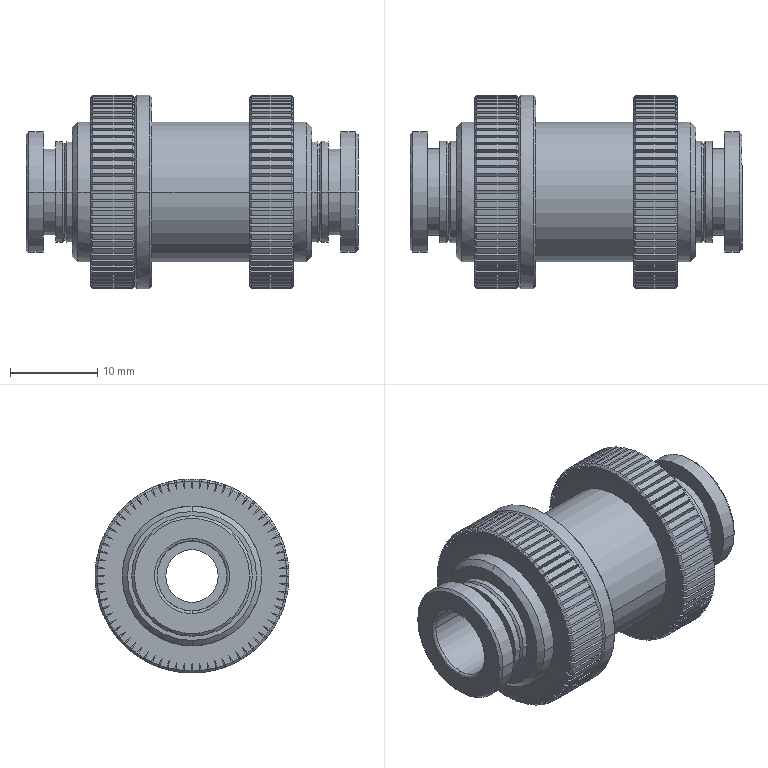Part | STEP file | CNTG-8 | 1 solid | 860 faces | box 38 x 22.2 x 22.2 mm | volume 6916 mm3 | plane 374 | cone 308 | cylinder 174 | spline 4 | commonest cylinder face diameters 22.2 x146 11.6 x8 16 x6 8 x4 9.9 x4 13.8 x4